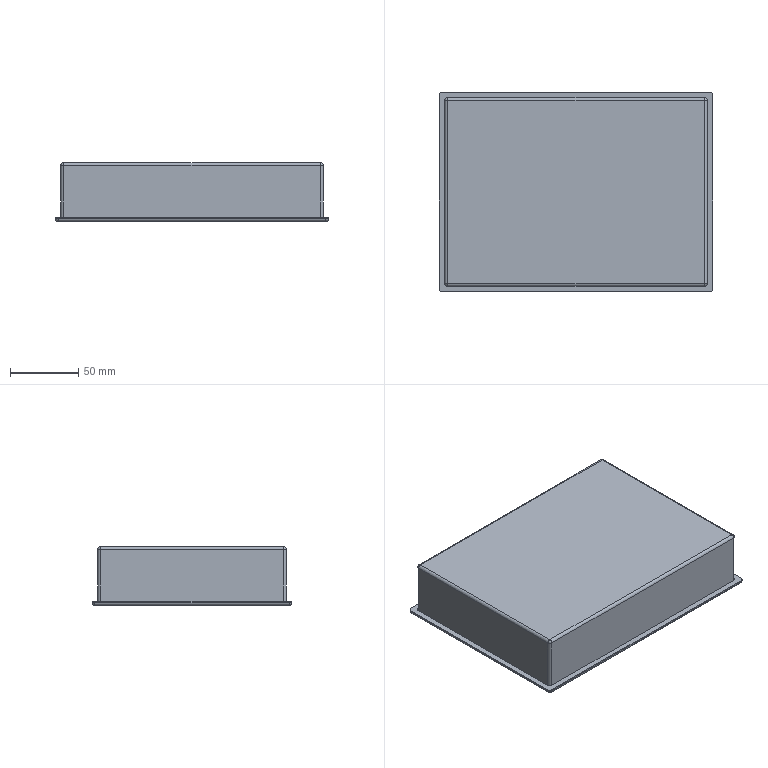Part | STEP file | QA-MT6070IH | 1 solid | 188 faces | box 200 x 146 x 43 mm | volume 1146130 mm3 | plane 98 | spline 66 | cylinder 16 | sphere 8 | commonest cylinder face diameters 4 x16